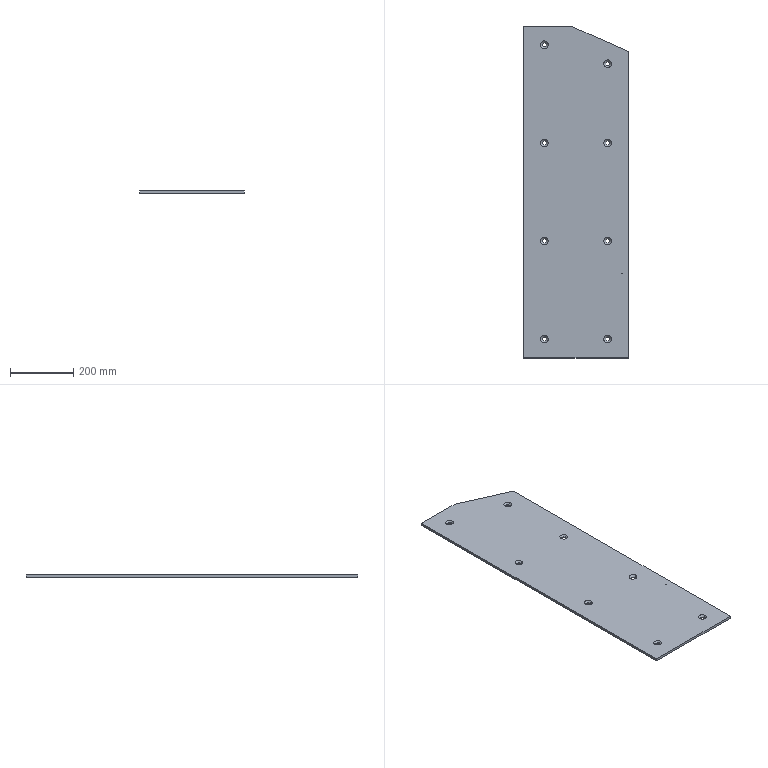Part | STEP file | Liner plate 1_Default<As machined> | 1 solid | 41 faces | box 330 x 1049 x 8 mm | volume 2695509 mm3 | cylinder 18 | cone 16 | plane 7 | commonest cylinder face diameters 13.5 x16 1.5 x2